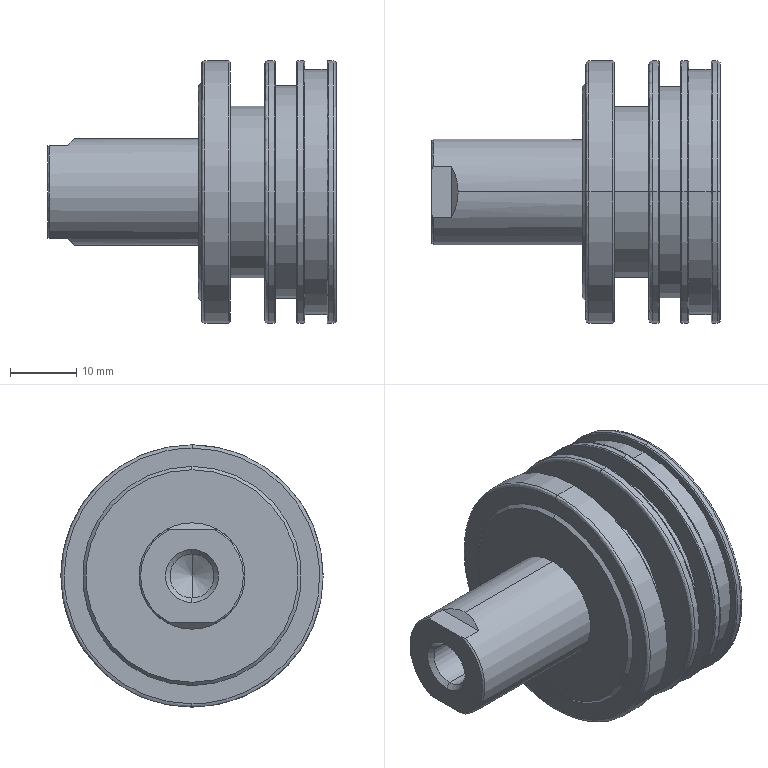Part | STEP file | 2_11 | 1 solid | 56 faces | box 43.5 x 39.5 x 39.5 mm | volume 23726 mm3 | cylinder 18 | spline 14 | plane 14 | cone 10 | commonest cylinder face diameters 39.5 x8 6.647 x2 16 x2 25.8 x2 32 x2 36.9 x2